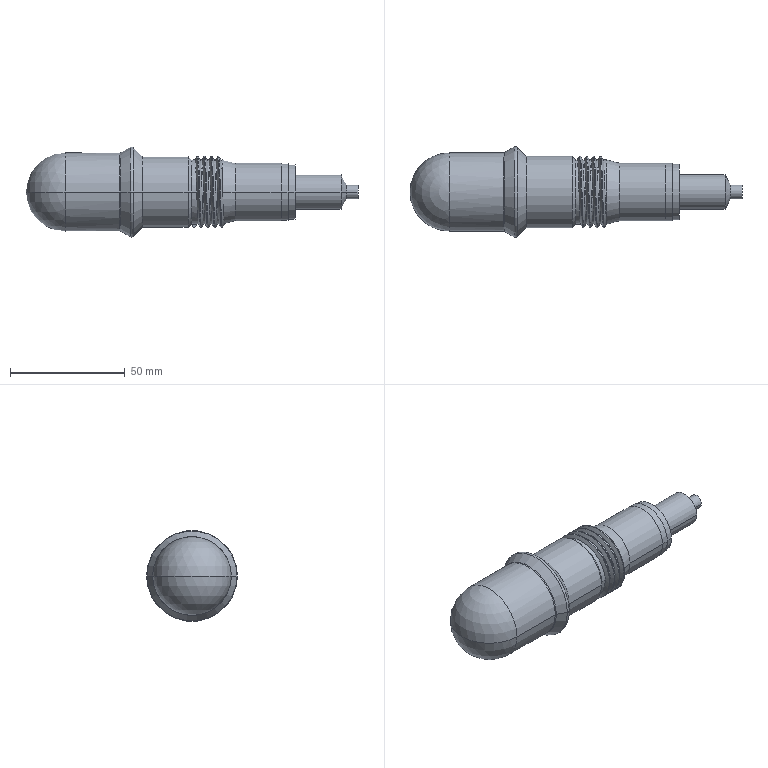Part | SolidWorks | features Fillet 1, Revolution 1, SweepThread 1 | 1 solid | 50 faces | box 144.393 x 39.501 x 39.501 mm | volume 86729 mm3 | cylinder 25 | cone 10 | plane 6 | torus 4 | spline 3 | sphere 2 | commonest cylinder face diameters 28 x11 6 x2 15 x2 24 x2 24.9 x2 25 x2